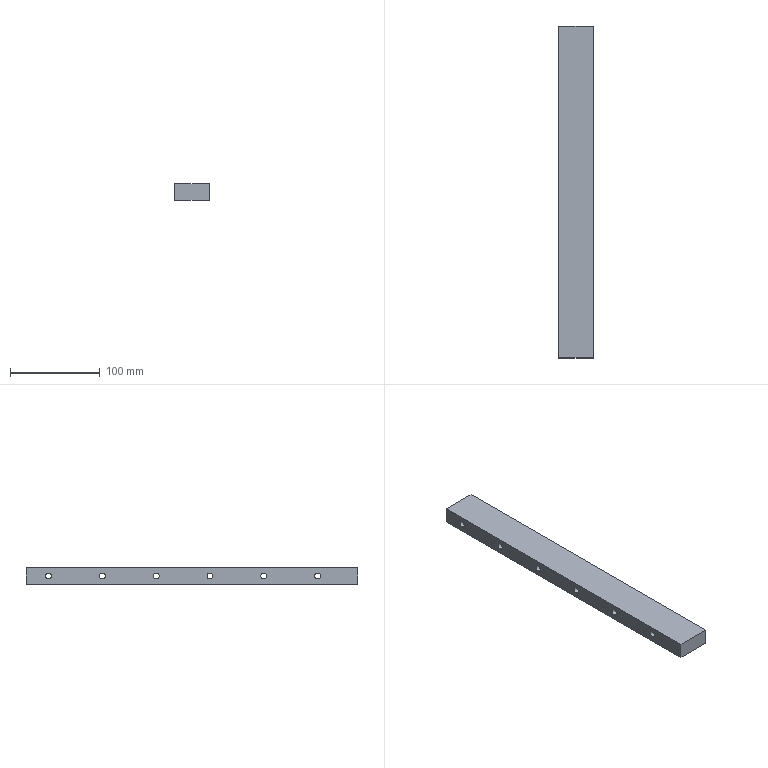Part | STEP file | PN_0039 spacer plate | 1 solid | 60 faces | box 39 x 370 x 18 mm | volume 248718 mm3 | cylinder 36 | cone 12 | plane 12 | commonest cylinder face diameters 3.3 x12 6.6 x12 11 x12